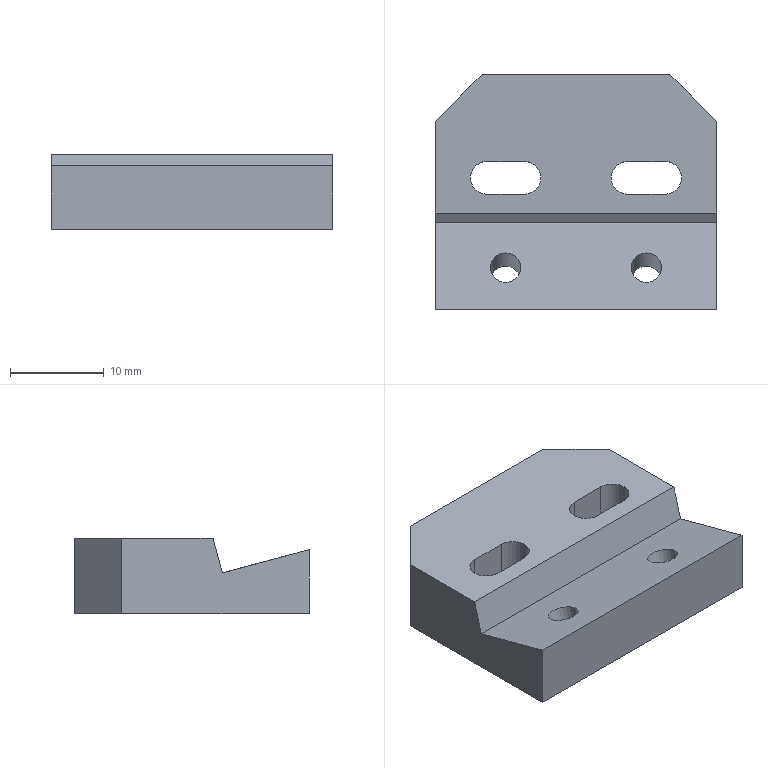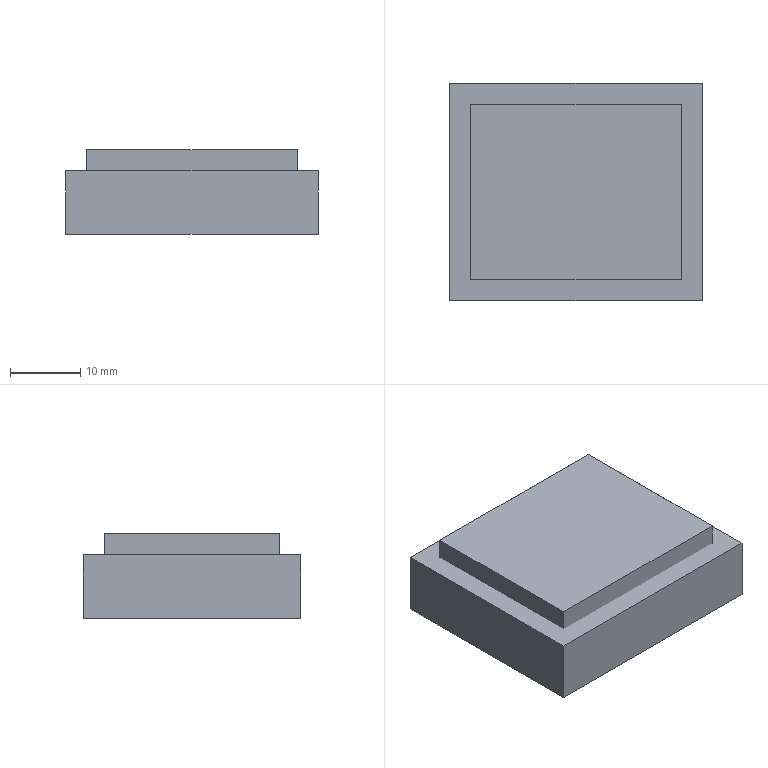CAM job | NX | 3+2 milling | part box 30 x 25 x 8 mm | stock box 36 x 31 x 12 mm
Tools:
number,name,description,diameter,corner_radius,flute_length,length,flutes
1,D63,Milling Tool-5 Parameters,63.0,0.0,50.0,75.0,2
9,D6A45,Milling Tool-5 Parameters,6.0,0.0,3.0,3.0,2
2,D10,Milling Tool-5 Parameters,10.0,0.0,50.0,75.0,2
4,D6,Milling Tool-5 Parameters,6.0,0.0,50.0,75.0,2
16,D3R0.5,Milling Tool-5 Parameters,3.0,0.5,50.0,75.0,2
8,D2,Milling Tool-5 Parameters,2.0,0.0,50.0,75.0,2
Operations:
program,operation,operation_type,tool,method,geometry_group,spindle_rpm,surface_speed,feed_per_tooth,feed_cut,feed_plunge,cut_length_mm,path_length_mm,cut_time_min,machine_time_min
1-35-30-12毛胚-桥板,FLOOR_WALL,VolumeBased25DMillingOperation,D63,METHOD,A,6500.0,0.0,0.0,1250.0,100.0,106.0,160.0,0.0848,0.0902
1-35-30-12毛胚-桥板,ADAPTIVE_MILLING,CavityMilling,D10,METHOD,A,7000.0,219.0,0.1429,2000.0,1000.0,736.99,806.99,0.37,0.377
1-35-30-12毛胚-桥板,ZLEVEL_PROFILE_COPY_COPY_1_COPY_COPY_COPY,ZLevelMilling,D10,METHOD,A,7000.0,65.0,0.1429,2000.0,1000.0,353.241,517.776,0.1811,0.1975
1-35-30-12毛胚-桥板,ZLEVEL_PROFILE_COPY_COPY_1_COPY,ZLevelMilling,D6,METHOD,A,6500.0,326.0,0.0769,1000.0,1000.0,129.592,202.592,0.1296,0.1369
1-35-30-12毛胚-桥板,ZLEVEL_PROFILE_COPY_COPY_1_COPY_COPY,ZLevelMilling,D3R0.5,METHOD,A,7000.0,65.0,0.1429,2000.0,1000.0,6139.986,6295.648,3.072,3.088
1-35-30-12毛胚-桥板,ZLEVEL_PROFILE_COPY_COPY_1_COPY_COPY_COPY_1,ZLevelMilling,D2,METHOD,A,7000.0,43.0,0.0714,1000.0,1000.0,2107.162,2250.279,2.107,2.122
1-35-30-12毛胚-桥板,ZLEVEL_PROFILE_COPY_1_COPY_COPY_COPY_COPY,ZLevelMilling,D6A45,METHOD,A,7000.0,131.0,0.0714,1000.0,1000.0,122.208,331.836,0.1222,0.1432
2-35-30-12毛胚-桥板,ZLEVEL_PROFILE_COPY_COPY_1_COPY_COPY_1,ZLevelMilling,D10,METHOD,B,6500.0,326.0,0.0769,1000.0,1000.0,49.046,106.046,0.049,0.0547
2-35-30-12毛胚-桥板,HOLE_MILLING,CylinderMilling,D2,METHOD,B,9500.0,59.0,0.0526,1000.0,100.0,578.153,723.665,0.5782,0.5927
2-35-30-12毛胚-桥板,ZLEVEL_PROFILE_COPY_1_COPY_COPY_COPY_COPY_COPY,ZLevelMilling,D6A45,METHOD,B,7000.0,131.0,0.0714,1000.0,1000.0,61.037,284.731,0.061,0.0834
3-35-30-12毛胚,FLOOR_WALL_COPY,VolumeBased25DMillingOperation,D63,METHOD,C,6500.0,0.0,0.0,1250.0,100.0,420.0,921.001,0.336,0.3861
3-35-30-12毛胚,ZLEVEL_PROFILE_COPY_1_COPY_COPY_COPY_COPY_COPY_1,ZLevelMilling,D6A45,METHOD,C,7000.0,131.0,0.0714,1000.0,1000.0,142.721,359.491,0.1427,0.1644